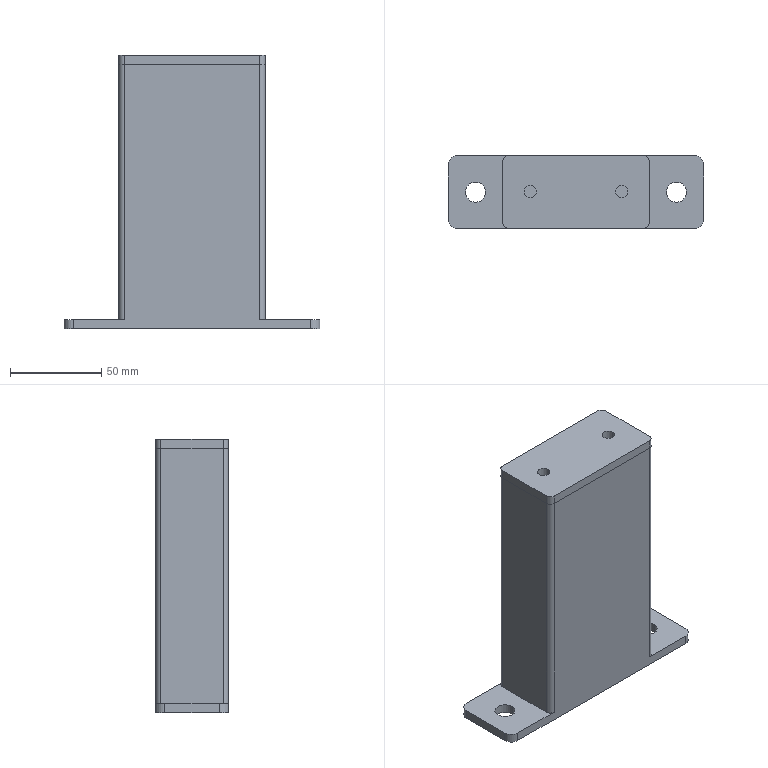Part | STEP file | 6-Slewing support rod_default<machined> | 2 solids | 45 faces | box 140 x 40 x 150 mm | volume 106539 mm3 | cylinder 24 | plane 21 | commonest cylinder face diameters 6 x8 2 x4 6.8 x4 10 x4 11 x4